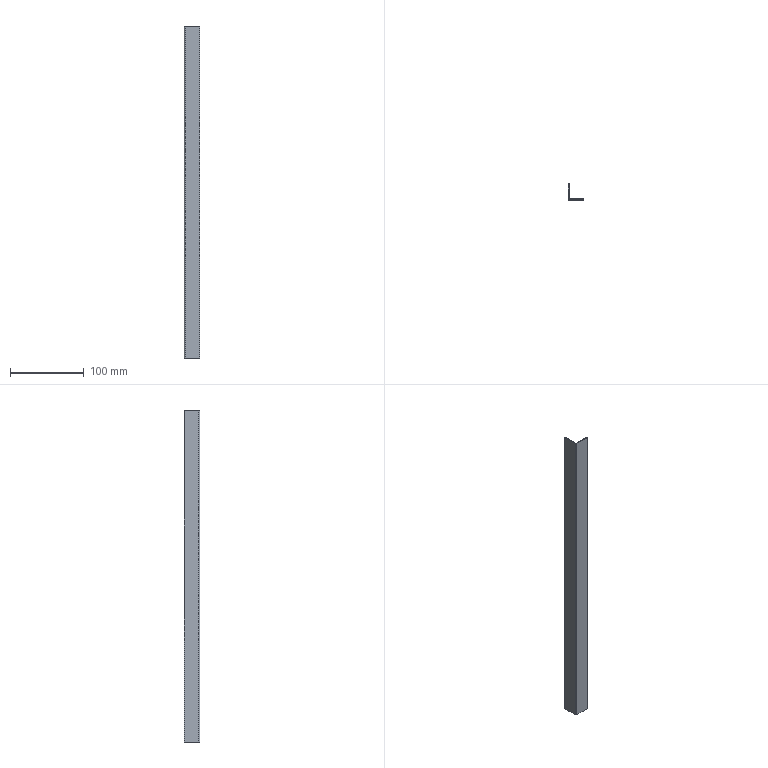Part | SolidWorks | features SplitBody 1 | 1 solid | 14 faces | box 21.5 x 21.5 x 450 mm | volume 27766 mm3 | plane 12 | cylinder 2 | commonest cylinder face diameters 0.2 x1 3.2 x1
STEP:
#1=CARTESIAN_POINT('',(-474.9,30.,185.));
#2=VERTEX_POINT('',#1);
#3=CARTESIAN_POINT('',(-474.9,28.5,185.));
#4=VERTEX_POINT('',#3);
#5=CARTESIAN_POINT('',(-474.9,30.,185.));
#6=DIRECTION('',(0.,-1.,0.));
#7=VECTOR('',#6,1000.);
#8=LINE('',#5,#7);
#9=EDGE_CURVE('',#2,#4,#8,.T.);
#10=ORIENTED_EDGE('',*,*,#9,.F.);
#11=CARTESIAN_POINT('',(-475.,30.1,185.));
#12=VERTEX_POINT('',#11);
#13=CARTESIAN_POINT('',(-474.9,30.1,185.));
#14=DIRECTION('',(0.,0.,-1.));
#15=DIRECTION('',(0.,-1.,0.));
#16=AXIS2_PLACEMENT_3D('',#13,#14,#15);
#17=CIRCLE('',#16,0.1);
#18=EDGE_CURVE('',#2,#12,#17,.T.);
#19=ORIENTED_EDGE('',*,*,#18,.T.);
#20=CARTESIAN_POINT('',(-476.5,30.1,185.));
#21=VERTEX_POINT('',#20);
#22=CARTESIAN_POINT('',(-476.5,30.1,185.));
#23=DIRECTION('',(1.,0.,0.));
#24=VECTOR('',#23,1000.);
#25=LINE('',#22,#24);
#26=EDGE_CURVE('',#21,#12,#25,.T.);
#27=ORIENTED_EDGE('',*,*,#26,.F.);
#28=CARTESIAN_POINT('',(-474.9,30.1,185.));
#29=DIRECTION('',(0.,0.,-1.));
#30=DIRECTION('',(-1.,0.,0.));
#31=AXIS2_PLACEMENT_3D('',#28,#29,#30);
#32=CIRCLE('',#31,1.6);
#33=EDGE_CURVE('',#4,#21,#32,.T.);
#34=ORIENTED_EDGE('',*,*,#33,.F.);
#35=EDGE_LOOP('',(#10,#19,#27,#34));
#36=FACE_OUTER_BOUND('',#35,.T.);
#37=CARTESIAN_POINT('',(-474.9,30.,185.));
#38=DIRECTION('',(0.,0.,1.));
#39=DIRECTION('',(0.,-1.,0.));
#40=AXIS2_PLACEMENT_3D('',#37,#38,#39);
#41=PLANE('',#40);
#42=ADVANCED_FACE('',(#36),#41,.T.);
#43=CARTESIAN_POINT('',(-455.,30.,185.));
#44=VERTEX_POINT('',#43);
#45=CARTESIAN_POINT('',(-455.,30.,185.));
#46=DIRECTION('',(-1.,0.,0.));
#47=VECTOR('',#46,1000.);
#48=LINE('',#45,#47);
#49=EDGE_CURVE('',#44,#2,#48,.T.);
#50=ORIENTED_EDGE('',*,*,#49,.T.);
#51=ORIENTED_EDGE('',*,*,#9,.T.);
#52=CARTESIAN_POINT('',(-455.,28.5,185.));
#53=VERTEX_POINT('',#52);
#54=CARTESIAN_POINT('',(-455.,28.5,185.));
#55=DIRECTION('',(-1.,0.,0.));
#56=VECTOR('',#55,1000.);
#57=LINE('',#54,#56);
#58=EDGE_CURVE('',#53,#4,#57,.T.);
#59=ORIENTED_EDGE('',*,*,#58,.F.);
#60=CARTESIAN_POINT('',(-455.,28.5,185.));
#61=DIRECTION('',(0.,1.,0.));
#62=VECTOR('',#61,1000.);
#63=LINE('',#60,#62);
#64=EDGE_CURVE('',#53,#44,#63,.T.);
#65=ORIENTED_EDGE('',*,*,#64,.T.);
#66=EDGE_LOOP('',(#50,#51,#59,#65));
#67=FACE_OUTER_BOUND('',#66,.T.);
#68=CARTESIAN_POINT('',(-476.5,30.1,185.));
#69=DIRECTION('',(0.,0.,1.));
#70=DIRECTION('',(0.,-1.,0.));
#71=AXIS2_PLACEMENT_3D('',#68,#69,#70);
#72=PLANE('',#71);
#73=ADVANCED_FACE('',(#67),#72,.T.);
#74=CARTESIAN_POINT('',(-476.5,50.,-265.));
#75=VERTEX_POINT('',#74);
#76=CARTESIAN_POINT('',(-476.5,30.1,-265.));
#77=VERTEX_POINT('',#76);
#78=CARTESIAN_POINT('',(-476.5,30.,-265.));
#79=DIRECTION('',(0.,-1.,0.));
#80=VECTOR('',#79,1000.);
#81=LINE('',#78,#80);
#82=EDGE_CURVE('',#75,#77,#81,.T.);
#83=ORIENTED_EDGE('',*,*,#82,.T.);
#84=CARTESIAN_POINT('',(-476.5,30.1,-295.406));
#85=DIRECTION('',(0.,0.,1.));
#86=VECTOR('',#85,1000.);
#87=LINE('',#84,#86);
#88=EDGE_CURVE('',#77,#21,#87,.T.);
#89=ORIENTED_EDGE('',*,*,#88,.T.);
#90=CARTESIAN_POINT('',(-476.5,50.,185.));
#91=VERTEX_POINT('',#90);
#92=CARTESIAN_POINT('',(-476.5,30.,185.));
#93=DIRECTION('',(0.,1.,0.));
#94=VECTOR('',#93,1000.);
#95=LINE('',#92,#94);
#96=EDGE_CURVE('',#21,#91,#95,.T.);
#97=ORIENTED_EDGE('',*,*,#96,.T.);
#98=CARTESIAN_POINT('',(-476.5,50.,-295.406));
#99=DIRECTION('',(0.,0.,1.));
#100=VECTOR('',#99,1000.);
#101=LINE('',#98,#100);
#102=EDGE_CURVE('',#75,#91,#101,.T.);
#103=ORIENTED_EDGE('',*,*,#102,.F.);
#104=EDGE_LOOP('',(#83,#89,#97,#103));
#105=FACE_OUTER_BOUND('',#104,.T.);
#106=CARTESIAN_POINT('',(-476.5,30.,-295.406));
#107=DIRECTION('',(1.,0.,0.));
#108=DIRECTION('',(0.,1.,0.));
#109=AXIS2_PLACEMENT_3D('',#106,#107,#108);
#110=PLANE('',#109);
#111=ADVANCED_FACE('',(#105),#110,.F.);
#112=CARTESIAN_POINT('',(-475.,50.,-265.));
#113=VERTEX_POINT('',#112);
#114=CARTESIAN_POINT('',(-475.,50.,185.));
#115=VERTEX_POINT('',#114);
#116=CARTESIAN_POINT('',(-475.,50.,-295.406));
#117=DIRECTION('',(0.,0.,1.));
#118=VECTOR('',#117,1000.);
#119=LINE('',#116,#118);
#120=EDGE_CURVE('',#113,#115,#119,.T.);
#121=ORIENTED_EDGE('',*,*,#120,.F.);
#122=CARTESIAN_POINT('',(-476.5,50.,-265.));
#123=DIRECTION('',(1.,0.,0.));
#124=VECTOR('',#123,1000.);
#125=LINE('',#122,#124);
#126=EDGE_CURVE('',#75,#113,#125,.T.);
#127=ORIENTED_EDGE('',*,*,#126,.F.);
#128=ORIENTED_EDGE('',*,*,#102,.T.);
#129=CARTESIAN_POINT('',(-475.,50.,185.));
#130=DIRECTION('',(-1.,0.,0.));
#131=VECTOR('',#130,1000.);
#132=LINE('',#129,#131);
#133=EDGE_CURVE('',#115,#91,#132,.T.);
#134=ORIENTED_EDGE('',*,*,#133,.F.);
#135=EDGE_LOOP('',(#121,#127,#128,#134));
#136=FACE_OUTER_BOUND('',#135,.T.);
#137=CARTESIAN_POINT('',(-475.,50.,-295.406));
#138=DIRECTION('',(0.,1.,0.));
#139=DIRECTION('',(0.,0.,1.));
#140=AXIS2_PLACEMENT_3D('',#137,#138,#139);
#141=PLANE('',#140);
#142=ADVANCED_FACE('',(#136),#141,.T.);
#143=CARTESIAN_POINT('',(-475.,30.1,-265.));
#144=VERTEX_POINT('',#143);
#145=CARTESIAN_POINT('',(-475.,30.1,-295.406));
#146=DIRECTION('',(0.,0.,1.));
#147=VECTOR('',#146,1000.);
#148=LINE('',#145,#147);
#149=EDGE_CURVE('',#144,#12,#148,.T.);
#150=ORIENTED_EDGE('',*,*,#149,.F.);
#151=CARTESIAN_POINT('',(-475.,30.,-265.));
#152=DIRECTION('',(0.,-1.,0.));
#153=VECTOR('',#152,1000.);
#154=LINE('',#151,#153);
#155=EDGE_CURVE('',#113,#144,#154,.T.);
#156=ORIENTED_EDGE('',*,*,#155,.F.);
#157=ORIENTED_EDGE('',*,*,#120,.T.);
#158=CARTESIAN_POINT('',(-475.,30.,185.));
#159=DIRECTION('',(0.,1.,0.));
#160=VECTOR('',#159,1000.);
#161=LINE('',#158,#160);
#162=EDGE_CURVE('',#12,#115,#161,.T.);
#163=ORIENTED_EDGE('',*,*,#162,.F.);
#164=EDGE_LOOP('',(#150,#156,#157,#163));
#165=FACE_OUTER_BOUND('',#164,.T.);
#166=CARTESIAN_POINT('',(-475.,30.,-295.406));
#167=DIRECTION('',(1.,0.,0.));
#168=DIRECTION('',(0.,1.,0.));
#169=AXIS2_PLACEMENT_3D('',#166,#167,#168);
#170=PLANE('',#169);
#171=ADVANCED_FACE('',(#165),#170,.T.);
#172=CARTESIAN_POINT('',(-474.9,30.,-265.));
#173=VERTEX_POINT('',#172);
#174=CARTESIAN_POINT('',(-474.9,30.,-295.406));
#175=DIRECTION('',(0.,0.,1.));
#176=VECTOR('',#175,1000.);
#177=LINE('',#174,#176);
#178=EDGE_CURVE('',#173,#2,#177,.T.);
#179=ORIENTED_EDGE('',*,*,#178,.F.);
#180=CARTESIAN_POINT('',(-474.9,30.1,-265.));
#181=DIRECTION('',(0.,0.,1.));
#182=DIRECTION('',(-1.,0.,0.));
#183=AXIS2_PLACEMENT_3D('',#180,#181,#182);
#184=CIRCLE('',#183,0.1);
#185=EDGE_CURVE('',#144,#173,#184,.T.);
#186=ORIENTED_EDGE('',*,*,#185,.F.);
#187=ORIENTED_EDGE('',*,*,#149,.T.);
#188=ORIENTED_EDGE('',*,*,#18,.F.);
#189=EDGE_LOOP('',(#179,#186,#187,#188));
#190=FACE_OUTER_BOUND('',#189,.T.);
#191=CARTESIAN_POINT('',(-474.9,30.1,-295.406));
#192=DIRECTION('',(0.,0.,1.));
#193=DIRECTION('',(0.,-1.,0.));
#194=AXIS2_PLACEMENT_3D('',#191,#192,#193);
#195=CYLINDRICAL_SURFACE('',#194,0.1);
#196=ADVANCED_FACE('',(#190),#195,.F.);
#197=CARTESIAN_POINT('',(-455.,30.,-265.));
#198=VERTEX_POINT('',#197);
#199=CARTESIAN_POINT('',(-455.,30.,-295.406));
#200=DIRECTION('',(0.,0.,1.));
#201=VECTOR('',#200,1000.);
#202=LINE('',#199,#201);
#203=EDGE_CURVE('',#198,#44,#202,.T.);
#204=ORIENTED_EDGE('',*,*,#203,.F.);
#205=CARTESIAN_POINT('',(-455.,30.,-265.));
#206=DIRECTION('',(1.,0.,0.));
#207=VECTOR('',#206,1000.);
#208=LINE('',#205,#207);
#209=EDGE_CURVE('',#173,#198,#208,.T.);
#210=ORIENTED_EDGE('',*,*,#209,.F.);
#211=ORIENTED_EDGE('',*,*,#178,.T.);
#212=ORIENTED_EDGE('',*,*,#49,.F.);
#213=EDGE_LOOP('',(#204,#210,#211,#212));
#214=FACE_OUTER_BOUND('',#213,.T.);
#215=CARTESIAN_POINT('',(-455.,30.,-295.406));
#216=DIRECTION('',(0.,1.,0.));
#217=DIRECTION('',(0.,0.,1.));
#218=AXIS2_PLACEMENT_3D('',#215,#216,#217);
#219=PLANE('',#218);
#220=ADVANCED_FACE('',(#214),#219,.T.);
#221=CARTESIAN_POINT('',(-455.,28.5,-265.));
#222=VERTEX_POINT('',#221);
#223=CARTESIAN_POINT('',(-455.,28.5,-295.406));
#224=DIRECTION('',(0.,0.,1.));
#225=VECTOR('',#224,1000.);
#226=LINE('',#223,#225);
#227=EDGE_CURVE('',#222,#53,#226,.T.);
#228=ORIENTED_EDGE('',*,*,#227,.F.);
#229=CARTESIAN_POINT('',(-455.,28.5,-265.));
#230=DIRECTION('',(0.,1.,0.));
#231=VECTOR('',#230,1000.);
#232=LINE('',#229,#231);
#233=EDGE_CURVE('',#222,#198,#232,.T.);
#234=ORIENTED_EDGE('',*,*,#233,.T.);
#235=ORIENTED_EDGE('',*,*,#203,.T.);
#236=ORIENTED_EDGE('',*,*,#64,.F.);
#237=EDGE_LOOP('',(#228,#234,#235,#236));
#238=FACE_OUTER_BOUND('',#237,.T.);
#239=CARTESIAN_POINT('',(-455.,28.5,-295.406));
#240=DIRECTION('',(1.,0.,0.));
#241=DIRECTION('',(0.,0.,-1.));
#242=AXIS2_PLACEMENT_3D('',#239,#240,#241);
#243=PLANE('',#242);
#244=ADVANCED_FACE('',(#238),#243,.T.);
#245=CARTESIAN_POINT('',(-474.9,28.5,-265.));
#246=VERTEX_POINT('',#245);
#247=CARTESIAN_POINT('',(-455.,28.5,-265.));
#248=DIRECTION('',(1.,0.,0.));
#249=VECTOR('',#248,1000.);
#250=LINE('',#247,#249);
#251=EDGE_CURVE('',#246,#222,#250,.T.);
#252=ORIENTED_EDGE('',*,*,#251,.T.);
#253=ORIENTED_EDGE('',*,*,#227,.T.);
#254=ORIENTED_EDGE('',*,*,#58,.T.);
#255=CARTESIAN_POINT('',(-474.9,28.5,-295.406));
#256=DIRECTION('',(0.,0.,1.));
#257=VECTOR('',#256,1000.);
#258=LINE('',#255,#257);
#259=EDGE_CURVE('',#246,#4,#258,.T.);
#260=ORIENTED_EDGE('',*,*,#259,.F.);
#261=EDGE_LOOP('',(#252,#253,#254,#260));
#262=FACE_OUTER_BOUND('',#261,.T.);
#263=CARTESIAN_POINT('',(-455.,28.5,-295.406));
#264=DIRECTION('',(0.,1.,0.));
#265=DIRECTION('',(0.,0.,1.));
#266=AXIS2_PLACEMENT_3D('',#263,#264,#265);
#267=PLANE('',#266);
#268=ADVANCED_FACE('',(#262),#267,.F.);
#269=CARTESIAN_POINT('',(-474.9,30.1,-265.));
#270=DIRECTION('',(0.,0.,1.));
#271=DIRECTION('',(1.,0.,0.));
#272=AXIS2_PLACEMENT_3D('',#269,#270,#271);
#273=CIRCLE('',#272,1.6);
#274=EDGE_CURVE('',#77,#246,#273,.T.);
#275=ORIENTED_EDGE('',*,*,#274,.T.);
#276=ORIENTED_EDGE('',*,*,#259,.T.);
#277=ORIENTED_EDGE('',*,*,#33,.T.);
#278=ORIENTED_EDGE('',*,*,#88,.F.);
#279=EDGE_LOOP('',(#275,#276,#277,#278));
#280=FACE_OUTER_BOUND('',#279,.T.);
#281=CARTESIAN_POINT('',(-474.9,30.1,-295.406));
#282=DIRECTION('',(0.,0.,1.));
#283=DIRECTION('',(0.,-1.,0.));
#284=AXIS2_PLACEMENT_3D('',#281,#282,#283);
#285=CYLINDRICAL_SURFACE('',#284,1.6);
#286=ADVANCED_FACE('',(#280),#285,.T.);
#287=ORIENTED_EDGE('',*,*,#96,.F.);
#288=ORIENTED_EDGE('',*,*,#26,.T.);
#289=ORIENTED_EDGE('',*,*,#162,.T.);
#290=ORIENTED_EDGE('',*,*,#133,.T.);
#291=EDGE_LOOP('',(#287,#288,#289,#290));
#292=FACE_OUTER_BOUND('',#291,.T.);
#293=CARTESIAN_POINT('',(-474.9,30.1,185.));
#294=DIRECTION('',(0.,0.,1.));
#295=DIRECTION('',(0.,1.,0.));
#296=AXIS2_PLACEMENT_3D('',#293,#294,#295);
#297=PLANE('',#296);
#298=ADVANCED_FACE('',(#292),#297,.T.);
#299=CARTESIAN_POINT('',(-476.5,30.1,-265.));
#300=DIRECTION('',(1.,0.,0.));
#301=VECTOR('',#300,1000.);
#302=LINE('',#299,#301);
#303=EDGE_CURVE('',#77,#144,#302,.T.);
#304=ORIENTED_EDGE('',*,*,#303,.F.);
#305=ORIENTED_EDGE('',*,*,#82,.F.);
#306=ORIENTED_EDGE('',*,*,#126,.T.);
#307=ORIENTED_EDGE('',*,*,#155,.T.);
#308=EDGE_LOOP('',(#304,#305,#306,#307));
#309=FACE_OUTER_BOUND('',#308,.T.);
#310=CARTESIAN_POINT('',(-476.5,30.,-265.));
#311=DIRECTION('',(0.,0.,1.));
#312=DIRECTION('',(0.,-1.,0.));
#313=AXIS2_PLACEMENT_3D('',#310,#311,#312);
#314=PLANE('',#313);
#315=ADVANCED_FACE('',(#309),#314,.F.);
#316=ORIENTED_EDGE('',*,*,#233,.F.);
#317=ORIENTED_EDGE('',*,*,#251,.F.);
#318=CARTESIAN_POINT('',(-474.9,28.5,-265.));
#319=DIRECTION('',(0.,1.,0.));
#320=VECTOR('',#319,1000.);
#321=LINE('',#318,#320);
#322=EDGE_CURVE('',#246,#173,#321,.T.);
#323=ORIENTED_EDGE('',*,*,#322,.T.);
#324=ORIENTED_EDGE('',*,*,#209,.T.);
#325=EDGE_LOOP('',(#316,#317,#323,#324));
#326=FACE_OUTER_BOUND('',#325,.T.);
#327=CARTESIAN_POINT('',(-455.,28.5,-265.));
#328=DIRECTION('',(0.,0.,1.));
#329=DIRECTION('',(1.,0.,0.));
#330=AXIS2_PLACEMENT_3D('',#327,#328,#329);
#331=PLANE('',#330);
#332=ADVANCED_FACE('',(#326),#331,.F.);
#333=ORIENTED_EDGE('',*,*,#185,.T.);
#334=ORIENTED_EDGE('',*,*,#322,.F.);
#335=ORIENTED_EDGE('',*,*,#274,.F.);
#336=ORIENTED_EDGE('',*,*,#303,.T.);
#337=EDGE_LOOP('',(#333,#334,#335,#336));
#338=FACE_OUTER_BOUND('',#337,.T.);
#339=CARTESIAN_POINT('',(-474.9,30.1,-265.));
#340=DIRECTION('',(0.,0.,-1.));
#341=DIRECTION('',(-1.,0.,0.));
#342=AXIS2_PLACEMENT_3D('',#339,#340,#341);
#343=PLANE('',#342);
#344=ADVANCED_FACE('',(#338),#343,.T.);
#345=CLOSED_SHELL('',(#42,#73,#111,#142,#171,#196,#220,#244,#268,#286,#298,#315,#332,#344));
#346=MANIFOLD_SOLID_BREP('',#345);
#347=CARTESIAN_POINT('',(0.,0.,0.));
#348=DIRECTION('',(0.,0.,1.));
#349=DIRECTION('',(1.,0.,0.));
#350=AXIS2_PLACEMENT_3D('',#347,#348,#349);
#351=(LENGTH_UNIT()NAMED_UNIT(*)SI_UNIT(.MILLI.,.METRE.));
#352=UNCERTAINTY_MEASURE_WITH_UNIT(LENGTH_MEASURE(0.00001),#351,'','');
#353=(NAMED_UNIT(*)PLANE_ANGLE_UNIT()SI_UNIT($,.RADIAN.));
#354=(NAMED_UNIT(*)SI_UNIT($,.STERADIAN.)SOLID_ANGLE_UNIT());
#355=(GEOMETRIC_REPRESENTATION_CONTEXT(3)GLOBAL_UNCERTAINTY_ASSIGNED_CONTEXT((#352))GLOBAL_UNIT_ASSIGNED_CONTEXT((#351,#353,#354))REPRESENTATION_CONTEXT('',''));
#356=ADVANCED_BREP_SHAPE_REPRESENTATION('',(#346,#350),#355);